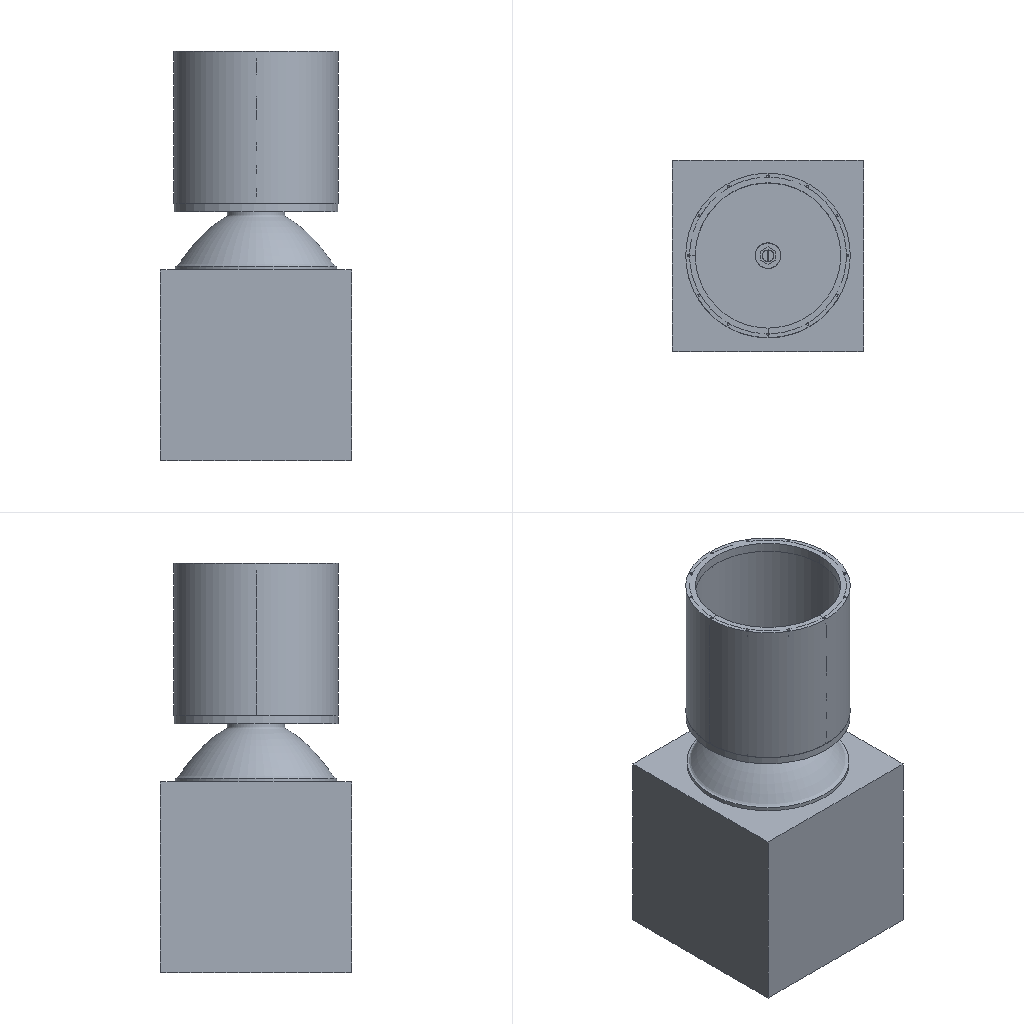Simulation study | abaqus
Set-up summary:
category,name,step,type,value,unit,region
solver,abaqus
solver,version,,,Abaqus/Explicit 2020
units,not stated in the deck,,not stated
analysis,deck,,transient,transient
load_step,Step-1,Step-1,transient,nlgeom=True
contact,interactions,,,general=1 pairs=0 ties=0
load_step,requested,,,1
mesh,nodes,,,58288
mesh,elements,,,51388
element_type,S3,,shell,1212
element_type,S4R,,shell,14189
element_type,C3D8R,,solid,35987
load,load commands in deck,,count,1
bc,support commands in deck,,count,4
material,JIEZHI,,in results
material,MATERIAL-1,,in results
check,setup vs results,,match,"per instance, exact: element labels, types and connectivity; labels of the nodes the elements use; coordinates of those nodes at SINGLE_PRECISION in 13 of 13 instance(s)"
Abaqus input file, long lists of numbers shortened:
*Heading
** Job name: Job-1 Model name: Model-1
** Generated by: Abaqus/CAE 2020
*Preprint, echo=NO, model=NO, history=NO, contact=NO
**
** PARTS
**
*Part, name=jiezhi
*Node
      1,           0.,        -500.,         500.
      2,           0.,        -480.,         500.
** (17574 more lines like these left out)
*Element, type=C3D8R
    1,   677,   678,   704,   703,     1,     2,    28,    27
    2,   678,   679,   705,   704,     2,     3,    29,    28
** (15623 more lines like these left out)
*Nset, nset=Set-1, generate
     1,  17576,      1
*Elset, elset=Set-1, generate
     1,  15625,      1
** Section: jiezhi
*Solid Section, elset=Set-1, material=jiezhi
,
*End Part
**
*Part, name=work-1
*Node
      1,           0.,        -215.,         200.
      2,           0.,        -215.,        -200.
** (4751 more lines like these left out)
*Element, type=S4R
  1,    1,  289, 1369,  358
  2,  289,  290, 1370, 1369
** (4659 more lines like these left out)
*Element, type=S3
2953,   22,   10, 3537
2954, 3539,   24, 3537
** (838 more lines like these left out)
*Nset, nset=Set-1
    1,    2,    3,    4,    5,    6,    7,    8,    9,   10,   11,   12,   13,   14,   15,   16
   17,   18,   19,   20,   21,   22,   23,   24,   25,   26,   27,   28,   29,   30,   31,   32
** (294 more lines like these left out)
*Elset, elset=Set-1
    1,    2,    3,    4,    5,    6,    7,    8,    9,   10,   11,   12,   13,   14,   15,   16
   17,   18,   19,   20,   21,   22,   23,   24,   25,   26,   27,   28,   29,   30,   31,   32
** (339 more lines like these left out)
*Nset, nset=Set-2, generate
    1,  4753,     1
*Elset, elset=Set-2, generate
    1,  5501,     1
** Section: Section-2
*Shell Section, elset=Set-2, material=Material-1
5., 5
*End Part
**
*Part, name=work-3
*Node
      1,  -14.187,  -4.87,       -359.5
      2,  -13.192,   -7.139,       -359.5
** (5733 more lines like these left out)
*Element, type=C3D8R
   1,  237,  238,  215,  195,   52,   53,   30,   10
   2,  278,  293,  322,  367,   93,  108,  137,  182
** (4948 more lines like these left out)
*Nset, nset=Set-1, generate
    1,  5735,     1
*Elset, elset=Set-1, generate
    1,  4950,     1
** Section: Section-1
*Solid Section, elset=Set-1, material=Material-1
,
*End Part
**
*Part, name=work-4
*Node
      1,           0.,         -15.,        -238.
      2,           0.,          15.,        -238.
** (3045 more lines like these left out)
*Element, type=S4R
  1,   1,  47, 639, 102
  2,  47,  48, 640, 639
** (3015 more lines like these left out)
*Element, type=S3
1463, 1891, 1892, 1823
1464, 1824, 1893, 1835
** (62 more lines like these left out)
*Nset, nset=Set-1
    1,    2,    3,    4,    5,    6,    7,    8,    9,   10,   11,   12,   13,   14,   15,   16
   17,   18,   19,   20,   21,   22,   23,   24,   25,   26,   27,   28,   29,   30,   31,   32
** (189 more lines like these left out)
*Elset, elset=Set-1
    1,    2,    3,    4,    5,    6,    7,    8,    9,   10,   11,   12,   13,   14,   15,   16
   17,   18,   19,   20,   21,   22,   23,   24,   25,   26,   27,   28,   29,   30,   31,   32
** (191 more lines like these left out)
*Nset, nset=Set-2, generate
    1,  3047,     1
*Elset, elset=Set-2, generate
    1,  3081,     1
** Section: Section-2
*Shell Section, elset=Set-2, material=Material-1
5., 5
*End Part
**
*Part, name=work-6
*Node
      1,         37.5,           0.,  -231.2
      2,        -37.5,           0.,  -231.2
** (4733 more lines like these left out)
*Element, type=S4R
 1,   1, 253, 300,   4
 2, 253, 254, 299, 300
** (4634 more lines like these left out)
*Element, type=S3
2572, 3271, 3270, 3253
2573, 3282, 3292, 3293
** (228 more lines like these left out)
*Nset, nset=Set-1, generate
    1,  4735,     1
*Elset, elset=Set-1, generate
    1,  4866,     1
** Section: Section-2
*Shell Section, elset=Set-1, material=Material-1
5., 5
*End Part
**
*Part, name=work-7
*Node
      1,  -77.6,           0.,  -233.152
      2,   77.6,           0.,  -233.152
** (1912 more lines like these left out)
*Element, type=S4R
  1,   1,  65, 641, 130
  2,  65,  66, 642, 641
** (1873 more lines like these left out)
*Element, type=S3
801, 1181, 1167, 1177
802, 1244, 1114, 1103
** (76 more lines like these left out)
*Nset, nset=Set-1, generate
    1,  1914,     1
*Elset, elset=Set-1, generate
    1,  1953,     1
** Section: Section-2
*Shell Section, elset=Set-1, material=Material-1
5., 5
*End Part
**
*Part, name=work-8
*Node
      1,         -18.,           0.,        -197.
      2,         -18.,           0.,  -194.2
** (9470 more lines like these left out)
*Element, type=C3D8R
   1,    3,   58, 1160,    2,  117, 1257, 4272,  282
   2,   58,   59, 1087, 1160, 1257, 1258, 4199, 4272
** (7486 more lines like these left out)
*Nset, nset=Set-1, generate
    1,  9472,     1
*Elset, elset=Set-1, generate
    1,  7488,     1
** Section: Section-1
*Solid Section, elset=Set-1, material=Material-1
,
*End Part
**
*Part, name=work-9
*Node
      1,          20.,   11.547,       -159.5
      2,           0.,   23.094,       -159.5
** (367 more lines like these left out)
*Element, type=C3D8R
  1,  44,   1,  33, 102, 167, 124, 156, 225
  2,  73,  72, 112, 121, 196, 195, 235, 244
** (174 more lines like these left out)
*Nset, nset=Set-1, generate
   1,  369,    1
*Elset, elset=Set-1, generate
   1,  176,    1
** Section: Section-1
*Solid Section, elset=Set-1, material=Material-1
,
*End Part
**
*Part, name=work-10
*Node
      1,         -20.,  -11.547,       -334.5
      2,           0.,  -23.094,       -334.5
** (367 more lines like these left out)
*Element, type=C3D8R
  1,  44,   1,  33, 103, 167, 124, 156, 226
  2,  73,  72, 113, 121, 196, 195, 236, 244
** (174 more lines like these left out)
*Nset, nset=Set-1, generate
   1,  369,    1
*Elset, elset=Set-1, generate
   1,  176,    1
** Section: Section-1
*Solid Section, elset=Set-1, material=Material-1
,
*End Part
**
*Part, name=work-11
*Node
      1,         -20.,  -11.547,       -351.5
      2,           0.,  -23.094,       -351.5
** (367 more lines like these left out)
*Element, type=C3D8R
  1,  44,   1,  33, 103, 167, 124, 156, 226
  2, 121, 113,  21, 112, 244, 236, 144, 235
** (174 more lines like these left out)
*Nset, nset=Set-1, generate
   1,  369,    1
*Elset, elset=Set-1, generate
   1,  176,    1
** Section: Section-1
*Solid Section, elset=Set-1, material=Material-1
,
*End Part
**
*Part, name=work-12
*Node
      1,         -20.,  -11.547,       -261.5
      2,           0.,  -23.094,       -261.5
** (367 more lines like these left out)
*Element, type=C3D8R
  1,  44,   1,  33, 102, 167, 124, 156, 225
  2, 121, 112,  21, 111, 244, 235, 144, 234
** (174 more lines like these left out)
*Nset, nset=Set-1, generate
   1,  369,    1
*Elset, elset=Set-1, generate
   1,  176,    1
** Section: Section-1
*Solid Section, elset=Set-1, material=Material-1
,
*End Part
**
*Part, name=work-13
*Node
      1,   16.627,    6.895,        -217.
      2,   16.627,    6.895,  -219.8
** (8218 more lines like these left out)
*Element, type=C3D8R
   1,    2,    3,   57, 1083,  240,  241, 1609, 3863
   2, 1039, 1070,   58,   59, 3819, 3850, 1610, 1611
** (6418 more lines like these left out)
*Nset, nset=Set-1, generate
    1,  8220,     1
*Elset, elset=Set-1, generate
    1,  6420,     1
** Section: Section-1
*Solid Section, elset=Set-1, material=Material-1
,
*End Part
**
*Part, name=yuan
*Node
      1,   56.944,  -48.809,   12.3
      2,   25.435,  -21.802,   12.3
** (1358 more lines like these left out)
*Element, type=C3D8R
  1,   29,   30,   31,   32,  427,  428,  337,  338
  2,  323,  322,   34,   35, 1075, 1074,  340,  341
** (798 more lines like these left out)
*Nset, nset=Set-1, generate
    1,  1360,     1
*Elset, elset=Set-1, generate
   1,  800,    1
** Section: Section-1
*Solid Section, elset=Set-1, material=Material-1
,
*End Part
**
**
** ASSEMBLY
**
*Assembly, name=Assembly
**
*Instance, name=work-1-1, part=work-1
*End Instance
**
*Instance, name=work-3-1, part=work-3
*End Instance
**
*Instance, name=work-4-1, part=work-4
*End Instance
**
*Instance, name=work-6-1, part=work-6
*End Instance
**
*Instance, name=work-7-1, part=work-7
*End Instance
**
*Instance, name=work-8-1, part=work-8
*End Instance
**
*Instance, name=work-9-1, part=work-9
*End Instance
**
*Instance, name=work-10-1, part=work-10
*End Instance
**
*Instance, name=work-11-1, part=work-11
*End Instance
**
*Instance, name=work-12-1, part=work-12
*End Instance
**
*Instance, name=work-13-1, part=work-13
*End Instance
**
*Instance, name=yuan-2, part=yuan
-2.69422295812418e-14,           0.,        -200.
-2.69422295812418e-14,           0.,        -200., -2.69422295812418e-14,           1.,        -200.,         180.
*End Instance
**
*Instance, name=jiezhi-1, part=jiezhi
       -250.,         250.,   -872.376
*End Instance
**
*Node
      1,           0., -1.28974378e-14,  -362.376
*Node
      2,           0., 1.31649528e-14,         200.
*Nset, nset=Set-3
 1,
*Nset, nset=Set-7
 2,
*Nset, nset=Set-8, instance=jiezhi-1
     1,    26,    27,    52,    53,    78,    79,   104,   105,   130,   131,   156,   157,   182,   183,   208
   209,   234,   235,   260,   261,   286,   287,   312,   313,   338,   339,   364,   365,   390,   391,   416
** (83 more lines like these left out)
*Elset, elset=Set-8, instance=jiezhi-1
     1,    25,    26,    50,    51,    75,    76,   100,   101,   125,   126,   150,   151,   175,   176,   200
   201,   225,   226,   250,   251,   275,   276,   300,   301,   325,   326,   350,   351,   375,   376,   400
** (77 more lines like these left out)
*Nset, nset=Set-9, instance=jiezhi-1
     1,     2,     3,     4,     5,     6,     7,     8,     9,    10,    11,    12,    13,    14,    15,    16
    17,    18,    19,    20,    21,    22,    23,    24,    25,    26,    27,    28,    29,    30,    31,    32
** (83 more lines like these left out)
*Elset, elset=Set-9, instance=jiezhi-1
     1,     2,     3,     4,     5,     6,     7,     8,     9,    10,    11,    12,    13,    14,    15,    16
    17,    18,    19,    20,    21,    22,    23,    24,    25,    26,    27,    28,    29,    30,    31,    32
** (77 more lines like these left out)
*Nset, nset=Set-10, instance=jiezhi-1
   651,   652,   653,   654,   655,   656,   657,   658,   659,   660,   661,   662,   663,   664,   665,   666
   667,   668,   669,   670,   671,   672,   673,   674,   675,   676,  1327,  1328,  1329,  1330,  1331,  1332
** (41 more lines like these left out)
*Elset, elset=Set-10, instance=jiezhi-1
   601,   602,   603,   604,   605,   606,   607,   608,   609,   610,   611,   612,   613,   614,   615,   616
   617,   618,   619,   620,   621,   622,   623,   624,   625,  1226,  1227,  1228,  1229,  1230,  1231,  1232
** (38 more lines like these left out)
*Nset, nset=m_Set-2
 1,
*Nset, nset=m_Set-6
 2,
*Elset, elset=_Surf-4_SPOS, internal, instance=work-7-1
  801,  802,  803,  804,  805,  806,  807,  808,  809,  810,  811,  812,  813,  814,  815,  816
  817,  818,  819,  820,  821,  822,  823,  824,  825,  826,  827,  828,  829,  830,  831,  832
** (25 more lines like these left out)
*Surface, type=ELEMENT, name=Surf-4
_Surf-4_SPOS, SPOS
*Elset, elset=_s_Surf-1_S2, internal, instance=work-3-1, generate
   1,  165,    1
*Surface, type=ELEMENT, name=s_Surf-1
_s_Surf-1_S2, S2
*Elset, elset=_s_Surf-3_SPOS, internal, instance=work-1-1
 3041, 3042, 3043, 3044, 3045, 3046, 3047, 3048, 3049, 3050, 3051, 3052, 3053, 3054, 3055, 3056
 3057, 3058, 3059, 3060, 3061, 3062, 3063, 3064, 3065, 3066, 3067, 3068, 3069, 3070, 3071, 3072
** (41 more lines like these left out)
*Surface, type=ELEMENT, name=s_Surf-3
_s_Surf-3_SPOS, SPOS
** Constraint: Constraint-1
*Coupling, constraint name=Constraint-1, ref node=m_Set-2, surface=s_Surf-1
*Kinematic
** Constraint: Constraint-2
*Coupling, constraint name=Constraint-2, ref node=m_Set-6, surface=s_Surf-3
*Kinematic
*End Assembly
*Amplitude, name=Amp-1, definition=PERIODIC
1,           6280.,              0.,              0.
             1.,              0.
**
** MATERIALS
**
*Material, name=Material-1
*Density
 7.8e-09,
*Elastic
210000., 0.3
*Plastic
350.,0.
*Material, name=jiezhi
*Density
 1e-09,
*Elastic
4., 0.4
**
** INTERACTION PROPERTIES
**
*Surface Interaction, name=IntProp-1
*Friction
 0.15,
*Surface Behavior, pressure-overclosure=HARD
** ----------------------------------------------------------------
**
** STEP: Step-1
**
*Step, name=Step-1, nlgeom=YES
*Dynamic, Explicit
, 0.01
*Bulk Viscosity
0.06, 1.2
** Mass Scaling: Semi-Automatic
**               Whole Model
*Fixed Mass Scaling, factor=500.
**
** BOUNDARY CONDITIONS
**
** Name: BC-1 Type: 对称/反对称/完全固定
*Boundary
Set-7, ENCASTRE
** Name: BC-2 Type: 位移/转角
*Boundary
Set-8, 2, 2
** Name: BC-3 Type: 位移/转角
*Boundary
Set-9, 1, 1
** Name: BC-4 Type: 位移/转角
*Boundary
Set-10, 3, 3
**
** LOADS
**
** Name: Load-2   Type: Pressure
*Dsload, amplitude=Amp-1
Surf-4, P, -10.
**
** INTERACTIONS
**
** Interaction: Int-1
*Contact, op=NEW
*Contact Inclusions, ALL EXTERIOR
*Contact Property Assignment
 ,  , IntProp-1
**
** OUTPUT REQUESTS
**
*Restart, write, number interval=1, time marks=NO
**
** FIELD OUTPUT: F-Output-1
**
*Output, field
*Node Output
A, CF, RF, RM, RT, U, V
*Element Output, directions=YES
E, EVF, LE, MISES, MISESMAX, PE, PEEQ, PEEQMAX, PEEQVAVG, PEMAG, PEVAVG, S, SEQUT, SVAVG, YIELDPOT
*Contact Output
CDISP, CSTRESS
**
** HISTORY OUTPUT: H-Output-2
**
*Output, history, time interval=2e-07
*Energy Output
ALLAE, ALLCD, ALLCW, ALLDC, ALLDMD, ALLFD, ALLIE, ALLKE, ALLMW, ALLPD, ALLPW, ALLSE, ALLVD, ALLWK, ETOTAL
**
** HISTORY OUTPUT: H-Output-1
**
*Node Output, nset=Set-7
RF1, RF2, RF3
*End Step
Results summary:
result,step,Step-1,completed,increments=26190 time=0.01/0.01
result,analysis,,,transient
result,last_loadstep,,,1
result,analysis steps,,count,1
result,primary field,,,"U, UR"
result,reaction total,,FX,23.512,model units
result,reaction total,,FY,39.612,model units
result,reaction total,,FZ,-2018.34,model units